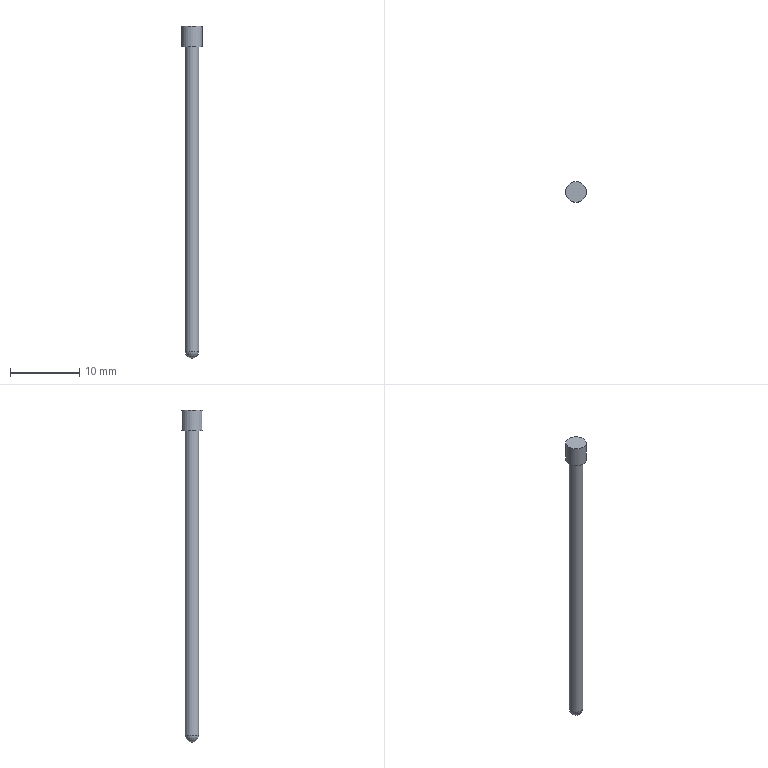Part | NX | features PG_666 2 | 1 solid | 6 faces | box 3 x 3 x 48 mm | volume 161.671 mm3 | plane 3 | cylinder 2 | torus 1 | commonest cylinder face diameters 2.001 x1 3 x1
STEP:
#1=CARTESIAN_POINT('',(2544.582,-830.019,851.716));
#2=VERTEX_POINT('',#1);
#3=CARTESIAN_POINT('',(2545.582,-830.019,851.716));
#4=DIRECTION('',(0.,0.,1.));
#5=DIRECTION('',(-1.,0.,0.));
#6=AXIS2_PLACEMENT_3D('',#3,#4,#5);
#7=CIRCLE('',#6,1.);
#8=EDGE_CURVE('',#2,#2,#7,.F.);
#9=ORIENTED_EDGE('',*,*,#8,.F.);
#10=EDGE_LOOP('',(#9));
#11=FACE_BOUND('',#10,.T.);
#12=CARTESIAN_POINT('',(2544.582,-830.019,895.716));
#13=VERTEX_POINT('',#12);
#14=CARTESIAN_POINT('',(2545.582,-830.019,895.716));
#15=DIRECTION('',(0.,0.,1.));
#16=DIRECTION('',(-1.,0.,0.));
#17=AXIS2_PLACEMENT_3D('',#14,#15,#16);
#18=CIRCLE('',#17,1.);
#19=EDGE_CURVE('',#13,#13,#18,.F.);
#20=ORIENTED_EDGE('',*,*,#19,.T.);
#21=EDGE_LOOP('',(#20));
#22=FACE_BOUND('',#21,.T.);
#23=CARTESIAN_POINT('',(2545.582,-830.019,855.716));
#24=DIRECTION('',(0.,0.,1.));
#25=DIRECTION('',(1.,0.,0.));
#26=AXIS2_PLACEMENT_3D('',#23,#24,#25);
#27=CYLINDRICAL_SURFACE('',#26,1.);
#28=ADVANCED_FACE('',(#11,#22),#27,.T.);
#29=CARTESIAN_POINT('',(2545.582,-830.019,850.716));
#30=VERTEX_POINT('',#29);
#31=CARTESIAN_POINT('',(2545.582,-830.019,850.716));
#32=DIRECTION('',(0.,0.,1.));
#33=DIRECTION('',(-1.,0.,0.));
#34=AXIS2_PLACEMENT_3D('',#31,#32,#33);
#35=CIRCLE('',#34,0.0005);
#36=EDGE_CURVE('',#30,#30,#35,.T.);
#37=ORIENTED_EDGE('',*,*,#36,.F.);
#38=EDGE_LOOP('',(#37));
#39=FACE_BOUND('',#38,.T.);
#40=CARTESIAN_POINT('',(2545.582,-830.019,850.716));
#41=DIRECTION('',(0.,0.,-1.));
#42=DIRECTION('',(-1.,0.,0.));
#43=AXIS2_PLACEMENT_3D('',#40,#41,#42);
#44=PLANE('',#43);
#45=ADVANCED_FACE('',(#39),#44,.T.);
#46=CARTESIAN_POINT('',(2547.082,-830.019,898.716));
#47=VERTEX_POINT('',#46);
#48=CARTESIAN_POINT('',(2545.582,-830.019,898.716));
#49=DIRECTION('',(0.,0.,1.));
#50=DIRECTION('',(1.,0.,0.));
#51=AXIS2_PLACEMENT_3D('',#48,#49,#50);
#52=CIRCLE('',#51,1.5);
#53=EDGE_CURVE('',#47,#47,#52,.T.);
#54=ORIENTED_EDGE('',*,*,#53,.T.);
#55=EDGE_LOOP('',(#54));
#56=FACE_BOUND('',#55,.T.);
#57=CARTESIAN_POINT('',(2545.582,-830.019,898.716));
#58=DIRECTION('',(0.,0.,1.));
#59=DIRECTION('',(1.,0.,0.));
#60=AXIS2_PLACEMENT_3D('',#57,#58,#59);
#61=PLANE('',#60);
#62=ADVANCED_FACE('',(#56),#61,.T.);
#63=ORIENTED_EDGE('',*,*,#19,.F.);
#64=EDGE_LOOP('',(#63));
#65=FACE_BOUND('',#64,.T.);
#66=CARTESIAN_POINT('',(2547.082,-830.019,895.716));
#67=VERTEX_POINT('',#66);
#68=CARTESIAN_POINT('',(2545.582,-830.019,895.716));
#69=DIRECTION('',(0.,0.,-1.));
#70=DIRECTION('',(1.,0.,0.));
#71=AXIS2_PLACEMENT_3D('',#68,#69,#70);
#72=CIRCLE('',#71,1.5);
#73=EDGE_CURVE('',#67,#67,#72,.T.);
#74=ORIENTED_EDGE('',*,*,#73,.T.);
#75=EDGE_LOOP('',(#74));
#76=FACE_BOUND('',#75,.T.);
#77=CARTESIAN_POINT('',(2545.582,-830.019,895.716));
#78=DIRECTION('',(0.,0.,-1.));
#79=DIRECTION('',(-1.,0.,0.));
#80=AXIS2_PLACEMENT_3D('',#77,#78,#79);
#81=PLANE('',#80);
#82=ADVANCED_FACE('',(#65,#76),#81,.T.);
#83=ORIENTED_EDGE('',*,*,#53,.F.);
#84=EDGE_LOOP('',(#83));
#85=FACE_BOUND('',#84,.T.);
#86=ORIENTED_EDGE('',*,*,#73,.F.);
#87=EDGE_LOOP('',(#86));
#88=FACE_BOUND('',#87,.T.);
#89=CARTESIAN_POINT('',(2545.582,-830.019,895.716));
#90=DIRECTION('',(0.,0.,1.));
#91=DIRECTION('',(1.,0.,0.));
#92=AXIS2_PLACEMENT_3D('',#89,#90,#91);
#93=CYLINDRICAL_SURFACE('',#92,1.5);
#94=ADVANCED_FACE('',(#85,#88),#93,.T.);
#95=ORIENTED_EDGE('',*,*,#36,.T.);
#96=EDGE_LOOP('',(#95));
#97=FACE_BOUND('',#96,.T.);
#98=ORIENTED_EDGE('',*,*,#8,.T.);
#99=EDGE_LOOP('',(#98));
#100=FACE_BOUND('',#99,.T.);
#101=CARTESIAN_POINT('',(2545.582,-830.019,851.716));
#102=DIRECTION('',(0.,0.,-1.));
#103=DIRECTION('',(-1.,0.,0.));
#104=AXIS2_PLACEMENT_3D('',#101,#102,#103);
#105=DEGENERATE_TOROIDAL_SURFACE('',#104,0.0005,1.,.T.);
#106=ADVANCED_FACE('',(#97,#100),#105,.T.);
#107=CLOSED_SHELL('',(#28,#45,#62,#82,#94,#106));
#108=MANIFOLD_SOLID_BREP('',#107);
#109=(LENGTH_UNIT()NAMED_UNIT(*)SI_UNIT(.MILLI.,.METRE.));
#110=UNCERTAINTY_MEASURE_WITH_UNIT(LENGTH_MEASURE(0.00001),#109,'','');
#111=(NAMED_UNIT(*)PLANE_ANGLE_UNIT()SI_UNIT($,.RADIAN.));
#112=(NAMED_UNIT(*)SI_UNIT($,.STERADIAN.)SOLID_ANGLE_UNIT());
#113=(GEOMETRIC_REPRESENTATION_CONTEXT(3)GLOBAL_UNCERTAINTY_ASSIGNED_CONTEXT((#110))GLOBAL_UNIT_ASSIGNED_CONTEXT((#109,#111,#112))REPRESENTATION_CONTEXT('',''));
#114=ADVANCED_BREP_SHAPE_REPRESENTATION('',(#108),#113);